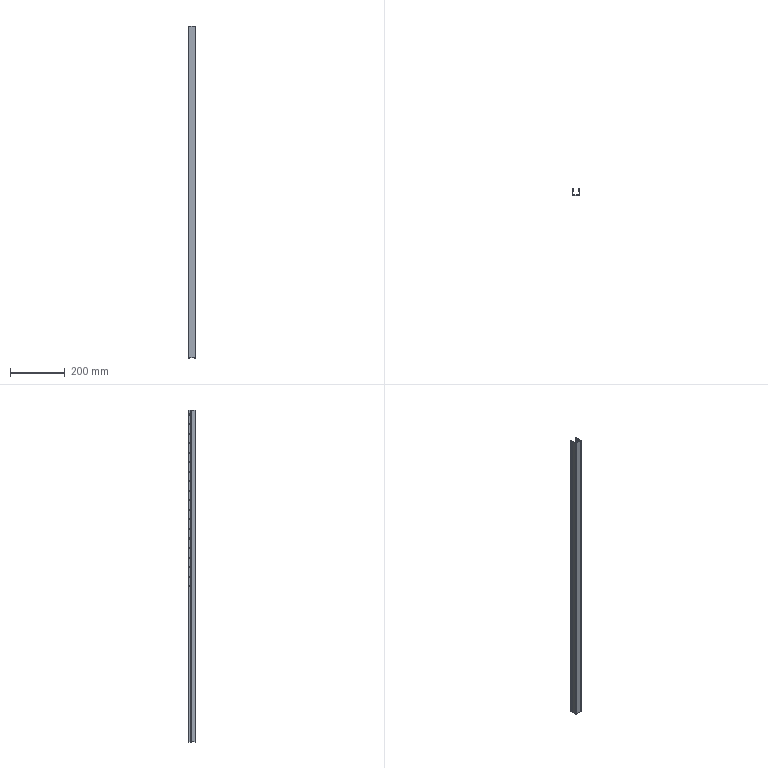Part | STEP file | GALVANIZED RAIL 24 | 1 solid | 120 faces | box 28.4 x 26.2 x 1218 mm | volume 121365 mm3 | cylinder 92 | plane 28 | commonest cylinder face diameters 4 x76 1.473 x8 3.873 x8